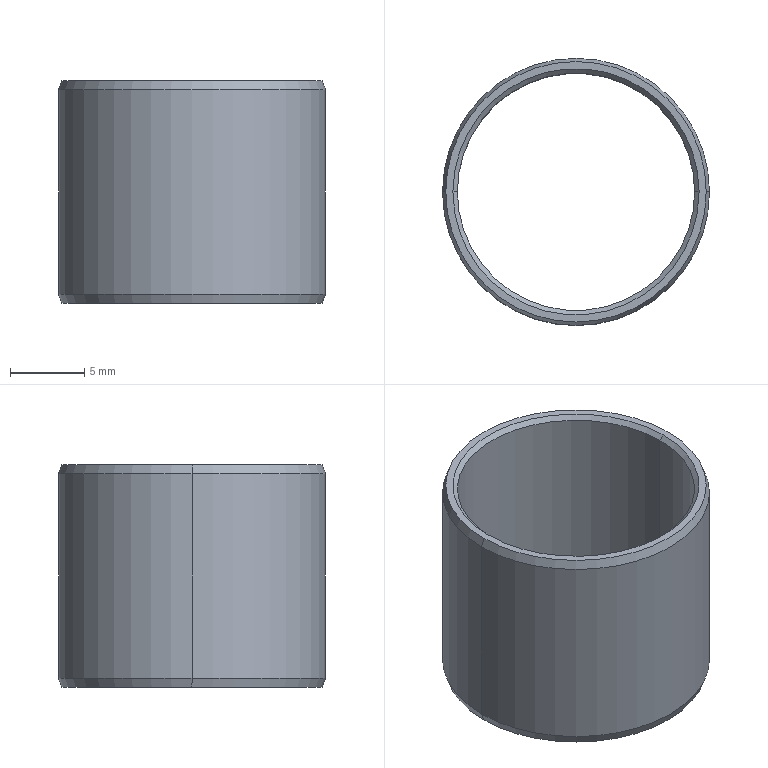Part | STEP file | SF-1 oil-free bearing 1615 | 1 solid | 14 faces | box 18 x 18 x 15 mm | volume 789.176 mm3 | cone 8 | cylinder 4 | plane 2 | commonest cylinder face diameters 16 x2 18 x2
STEP:
#1=CARTESIAN_POINT('',(0.,0.,0.));
#2=DIRECTION('',(0.,0.,1.));
#3=DIRECTION('',(1.,0.,0.));
#4=AXIS2_PLACEMENT_3D('',#1,#2,#3);
#5=CARTESIAN_POINT('',(-8.782,0.,0.));
#6=VERTEX_POINT('',#5);
#7=CARTESIAN_POINT('',(8.782,0.,0.));
#8=VERTEX_POINT('',#7);
#9=CARTESIAN_POINT('',(0.,0.,0.));
#10=DIRECTION('',(0.,0.,-1.));
#11=DIRECTION('',(1.,0.,0.));
#12=AXIS2_PLACEMENT_3D('',#9,#10,#11);
#13=CIRCLE('',#12,8.782);
#14=CARTESIAN_POINT('',(0.,0.,0.6));
#15=DIRECTION('',(0.,0.,1.));
#16=DIRECTION('',(1.,0.,0.));
#17=AXIS2_PLACEMENT_3D('',#14,#15,#16);
#18=CONICAL_SURFACE('',#17,9.,0.3491);
#19=CARTESIAN_POINT('',(6.283,-0.6));
#20=DIRECTION('',(-1.,0.));
#21=VECTOR('',#20,1.);
#22=LINE('',#19,#21);
#23=(GEOMETRIC_REPRESENTATION_CONTEXT(2)PARAMETRIC_REPRESENTATION_CONTEXT()REPRESENTATION_CONTEXT('',''));
#24=DEFINITIONAL_REPRESENTATION('',(#22),#23);
#25=PCURVE('',#18,#24);
#26=CARTESIAN_POINT('',(0.,0.,0.));
#27=DIRECTION('',(0.,0.,1.));
#28=DIRECTION('',(1.,0.,0.));
#29=AXIS2_PLACEMENT_3D('',#26,#27,#28);
#30=PLANE('',#29);
#31=CARTESIAN_POINT('',(8.782,0.));
#32=CARTESIAN_POINT('',(8.782,-15.21));
#33=CARTESIAN_POINT('',(-4.391,-7.605));
#34=CARTESIAN_POINT('',(-17.563,0.));
#35=CARTESIAN_POINT('',(-4.391,7.605));
#36=CARTESIAN_POINT('',(8.782,15.21));
#37=CARTESIAN_POINT('',(8.782,0.));
#38=(BOUNDED_CURVE()B_SPLINE_CURVE(2,(#31,#32,#33,#34,#35,#36,#37),.UNSPECIFIED.,.T.,.F.)B_SPLINE_CURVE_WITH_KNOTS((1,2,2,2,2,1),(-2.094,0.,2.094,4.189,6.283,8.378),.UNSPECIFIED.)CURVE()GEOMETRIC_REPRESENTATION_ITEM()RATIONAL_B_SPLINE_CURVE((1.,0.5,1.,0.5,1.,0.5,1.))REPRESENTATION_ITEM(''));
#39=(GEOMETRIC_REPRESENTATION_CONTEXT(2)PARAMETRIC_REPRESENTATION_CONTEXT()REPRESENTATION_CONTEXT('',''));
#40=DEFINITIONAL_REPRESENTATION('',(#38),#39);
#41=PCURVE('',#30,#40);
#42=SURFACE_CURVE('',#13,(#25,#41),.PCURVE_S1.);
#43=EDGE_CURVE('',#6,#8,#42,.T.);
#44=ORIENTED_EDGE('',*,*,#43,.F.);
#45=CARTESIAN_POINT('',(-9.,0.,0.6));
#46=VERTEX_POINT('',#45);
#47=CARTESIAN_POINT('',(-9.,0.,0.6));
#48=DIRECTION('',(-0.342,0.,0.9397));
#49=VECTOR('',#48,1.);
#50=LINE('',#47,#49);
#51=CARTESIAN_POINT('',(3.142,0.));
#52=DIRECTION('',(0.,1.));
#53=VECTOR('',#52,1.);
#54=LINE('',#51,#53);
#55=(GEOMETRIC_REPRESENTATION_CONTEXT(2)PARAMETRIC_REPRESENTATION_CONTEXT()REPRESENTATION_CONTEXT('',''));
#56=DEFINITIONAL_REPRESENTATION('',(#54),#55);
#57=PCURVE('',#18,#56);
#58=CARTESIAN_POINT('',(0.,0.,0.6));
#59=DIRECTION('',(0.,0.,1.));
#60=DIRECTION('',(1.,0.,0.));
#61=AXIS2_PLACEMENT_3D('',#58,#59,#60);
#62=CONICAL_SURFACE('',#61,9.,0.3491);
#63=CARTESIAN_POINT('',(3.142,0.));
#64=DIRECTION('',(0.,1.));
#65=VECTOR('',#64,1.);
#66=LINE('',#63,#65);
#67=(GEOMETRIC_REPRESENTATION_CONTEXT(2)PARAMETRIC_REPRESENTATION_CONTEXT()REPRESENTATION_CONTEXT('',''));
#68=DEFINITIONAL_REPRESENTATION('',(#66),#67);
#69=PCURVE('',#62,#68);
#70=SURFACE_CURVE('',#50,(#57,#69),.PCURVE_S1.);
#71=EDGE_CURVE('',#6,#46,#70,.T.);
#72=ORIENTED_EDGE('',*,*,#71,.T.);
#73=CARTESIAN_POINT('',(9.,0.,0.6));
#74=VERTEX_POINT('',#73);
#75=CARTESIAN_POINT('',(0.,0.,0.6));
#76=DIRECTION('',(0.,0.,1.));
#77=DIRECTION('',(1.,0.,0.));
#78=AXIS2_PLACEMENT_3D('',#75,#76,#77);
#79=CIRCLE('',#78,9.);
#80=CARTESIAN_POINT('',(0.,0.));
#81=DIRECTION('',(1.,0.));
#82=VECTOR('',#81,1.);
#83=LINE('',#80,#82);
#84=(GEOMETRIC_REPRESENTATION_CONTEXT(2)PARAMETRIC_REPRESENTATION_CONTEXT()REPRESENTATION_CONTEXT('',''));
#85=DEFINITIONAL_REPRESENTATION('',(#83),#84);
#86=PCURVE('',#18,#85);
#87=CARTESIAN_POINT('',(0.,0.,15.));
#88=DIRECTION('',(0.,0.,-1.));
#89=DIRECTION('',(-1.,0.,0.));
#90=AXIS2_PLACEMENT_3D('',#87,#88,#89);
#91=CYLINDRICAL_SURFACE('',#90,9.);
#92=CARTESIAN_POINT('',(3.142,14.4));
#93=DIRECTION('',(-1.,0.));
#94=VECTOR('',#93,1.);
#95=LINE('',#92,#94);
#96=(GEOMETRIC_REPRESENTATION_CONTEXT(2)PARAMETRIC_REPRESENTATION_CONTEXT()REPRESENTATION_CONTEXT('',''));
#97=DEFINITIONAL_REPRESENTATION('',(#95),#96);
#98=PCURVE('',#91,#97);
#99=SURFACE_CURVE('',#79,(#86,#98),.PCURVE_S1.);
#100=EDGE_CURVE('',#74,#46,#99,.T.);
#101=ORIENTED_EDGE('',*,*,#100,.F.);
#102=CARTESIAN_POINT('',(9.,0.,0.6));
#103=DIRECTION('',(0.342,0.,0.9397));
#104=VECTOR('',#103,1.);
#105=LINE('',#102,#104);
#106=CARTESIAN_POINT('',(0.,0.));
#107=DIRECTION('',(0.,1.));
#108=VECTOR('',#107,1.);
#109=LINE('',#106,#108);
#110=(GEOMETRIC_REPRESENTATION_CONTEXT(2)PARAMETRIC_REPRESENTATION_CONTEXT()REPRESENTATION_CONTEXT('',''));
#111=DEFINITIONAL_REPRESENTATION('',(#109),#110);
#112=PCURVE('',#18,#111);
#113=CARTESIAN_POINT('',(6.283,0.));
#114=DIRECTION('',(0.,1.));
#115=VECTOR('',#114,1.);
#116=LINE('',#113,#115);
#117=(GEOMETRIC_REPRESENTATION_CONTEXT(2)PARAMETRIC_REPRESENTATION_CONTEXT()REPRESENTATION_CONTEXT('',''));
#118=DEFINITIONAL_REPRESENTATION('',(#116),#117);
#119=PCURVE('',#62,#118);
#120=SURFACE_CURVE('',#105,(#112,#119),.PCURVE_S1.);
#121=EDGE_CURVE('',#8,#74,#120,.T.);
#122=ORIENTED_EDGE('',*,*,#121,.F.);
#123=EDGE_LOOP('',(#44,#72,#101,#122));
#124=FACE_BOUND('',#123,.T.);
#125=ADVANCED_FACE('',(#124),#18,.T.);
#126=CARTESIAN_POINT('',(8.782,0.,15.));
#127=VERTEX_POINT('',#126);
#128=CARTESIAN_POINT('',(-8.782,0.,15.));
#129=VERTEX_POINT('',#128);
#130=CARTESIAN_POINT('',(0.,0.,15.));
#131=DIRECTION('',(0.,0.,1.));
#132=DIRECTION('',(1.,0.,0.));
#133=AXIS2_PLACEMENT_3D('',#130,#131,#132);
#134=CIRCLE('',#133,8.782);
#135=CARTESIAN_POINT('',(0.,0.,15.));
#136=DIRECTION('',(0.,0.,-1.));
#137=DIRECTION('',(-1.,0.,0.));
#138=AXIS2_PLACEMENT_3D('',#135,#136,#137);
#139=CONICAL_SURFACE('',#138,8.782,0.3491);
#140=CARTESIAN_POINT('',(3.142,0.));
#141=DIRECTION('',(-1.,0.));
#142=VECTOR('',#141,1.);
#143=LINE('',#140,#142);
#144=(GEOMETRIC_REPRESENTATION_CONTEXT(2)PARAMETRIC_REPRESENTATION_CONTEXT()REPRESENTATION_CONTEXT('',''));
#145=DEFINITIONAL_REPRESENTATION('',(#143),#144);
#146=PCURVE('',#139,#145);
#147=CARTESIAN_POINT('',(0.,0.,15.));
#148=DIRECTION('',(0.,0.,1.));
#149=DIRECTION('',(1.,0.,0.));
#150=AXIS2_PLACEMENT_3D('',#147,#148,#149);
#151=PLANE('',#150);
#152=CARTESIAN_POINT('',(0.,0.));
#153=DIRECTION('',(1.,0.));
#154=AXIS2_PLACEMENT_2D('',#152,#153);
#155=CIRCLE('',#154,8.782);
#156=(GEOMETRIC_REPRESENTATION_CONTEXT(2)PARAMETRIC_REPRESENTATION_CONTEXT()REPRESENTATION_CONTEXT('',''));
#157=DEFINITIONAL_REPRESENTATION('',(#155),#156);
#158=PCURVE('',#151,#157);
#159=SURFACE_CURVE('',#134,(#146,#158),.PCURVE_S1.);
#160=EDGE_CURVE('',#127,#129,#159,.T.);
#161=ORIENTED_EDGE('',*,*,#160,.F.);
#162=CARTESIAN_POINT('',(9.,0.,14.4));
#163=VERTEX_POINT('',#162);
#164=CARTESIAN_POINT('',(8.782,0.,15.));
#165=DIRECTION('',(0.342,0.,-0.9397));
#166=VECTOR('',#165,1.);
#167=LINE('',#164,#166);
#168=CARTESIAN_POINT('',(3.142,0.));
#169=DIRECTION('',(0.,1.));
#170=VECTOR('',#169,1.);
#171=LINE('',#168,#170);
#172=(GEOMETRIC_REPRESENTATION_CONTEXT(2)PARAMETRIC_REPRESENTATION_CONTEXT()REPRESENTATION_CONTEXT('',''));
#173=DEFINITIONAL_REPRESENTATION('',(#171),#172);
#174=PCURVE('',#139,#173);
#175=CARTESIAN_POINT('',(0.,0.,15.));
#176=DIRECTION('',(0.,0.,-1.));
#177=DIRECTION('',(-1.,0.,0.));
#178=AXIS2_PLACEMENT_3D('',#175,#176,#177);
#179=CONICAL_SURFACE('',#178,8.782,0.3491);
#180=CARTESIAN_POINT('',(3.142,0.));
#181=DIRECTION('',(0.,1.));
#182=VECTOR('',#181,1.);
#183=LINE('',#180,#182);
#184=(GEOMETRIC_REPRESENTATION_CONTEXT(2)PARAMETRIC_REPRESENTATION_CONTEXT()REPRESENTATION_CONTEXT('',''));
#185=DEFINITIONAL_REPRESENTATION('',(#183),#184);
#186=PCURVE('',#179,#185);
#187=SURFACE_CURVE('',#167,(#174,#186),.PCURVE_S1.);
#188=EDGE_CURVE('',#127,#163,#187,.T.);
#189=ORIENTED_EDGE('',*,*,#188,.T.);
#190=CARTESIAN_POINT('',(-9.,0.,14.4));
#191=VERTEX_POINT('',#190);
#192=CARTESIAN_POINT('',(0.,0.,14.4));
#193=DIRECTION('',(0.,0.,-1.));
#194=DIRECTION('',(1.,0.,0.));
#195=AXIS2_PLACEMENT_3D('',#192,#193,#194);
#196=CIRCLE('',#195,9.);
#197=CARTESIAN_POINT('',(-3.142,0.6));
#198=DIRECTION('',(1.,0.));
#199=VECTOR('',#198,1.);
#200=LINE('',#197,#199);
#201=(GEOMETRIC_REPRESENTATION_CONTEXT(2)PARAMETRIC_REPRESENTATION_CONTEXT()REPRESENTATION_CONTEXT('',''));
#202=DEFINITIONAL_REPRESENTATION('',(#200),#201);
#203=PCURVE('',#139,#202);
#204=CARTESIAN_POINT('',(-3.142,0.6));
#205=DIRECTION('',(1.,0.));
#206=VECTOR('',#205,1.);
#207=LINE('',#204,#206);
#208=(GEOMETRIC_REPRESENTATION_CONTEXT(2)PARAMETRIC_REPRESENTATION_CONTEXT()REPRESENTATION_CONTEXT('',''));
#209=DEFINITIONAL_REPRESENTATION('',(#207),#208);
#210=PCURVE('',#91,#209);
#211=SURFACE_CURVE('',#196,(#203,#210),.PCURVE_S1.);
#212=EDGE_CURVE('',#191,#163,#211,.T.);
#213=ORIENTED_EDGE('',*,*,#212,.F.);
#214=CARTESIAN_POINT('',(-8.782,0.,15.));
#215=DIRECTION('',(-0.342,0.,-0.9397));
#216=VECTOR('',#215,1.);
#217=LINE('',#214,#216);
#218=CARTESIAN_POINT('',(0.,0.));
#219=DIRECTION('',(0.,1.));
#220=VECTOR('',#219,1.);
#221=LINE('',#218,#220);
#222=(GEOMETRIC_REPRESENTATION_CONTEXT(2)PARAMETRIC_REPRESENTATION_CONTEXT()REPRESENTATION_CONTEXT('',''));
#223=DEFINITIONAL_REPRESENTATION('',(#221),#222);
#224=PCURVE('',#139,#223);
#225=CARTESIAN_POINT('',(6.283,0.));
#226=DIRECTION('',(0.,1.));
#227=VECTOR('',#226,1.);
#228=LINE('',#225,#227);
#229=(GEOMETRIC_REPRESENTATION_CONTEXT(2)PARAMETRIC_REPRESENTATION_CONTEXT()REPRESENTATION_CONTEXT('',''));
#230=DEFINITIONAL_REPRESENTATION('',(#228),#229);
#231=PCURVE('',#179,#230);
#232=SURFACE_CURVE('',#217,(#224,#231),.PCURVE_S1.);
#233=EDGE_CURVE('',#129,#191,#232,.T.);
#234=ORIENTED_EDGE('',*,*,#233,.F.);
#235=EDGE_LOOP('',(#161,#189,#213,#234));
#236=FACE_BOUND('',#235,.T.);
#237=ADVANCED_FACE('',(#236),#139,.T.);
#238=CARTESIAN_POINT('',(8.,0.,14.7));
#239=VERTEX_POINT('',#238);
#240=CARTESIAN_POINT('',(8.3,0.,15.));
#241=VERTEX_POINT('',#240);
#242=CARTESIAN_POINT('',(8.,0.,14.7));
#243=DIRECTION('',(0.7071,0.,0.7071));
#244=VECTOR('',#243,1.);
#245=LINE('',#242,#244);
#246=CARTESIAN_POINT('',(0.,0.,14.7));
#247=DIRECTION('',(0.,0.,1.));
#248=DIRECTION('',(1.,0.,0.));
#249=AXIS2_PLACEMENT_3D('',#246,#247,#248);
#250=CONICAL_SURFACE('',#249,8.,0.7854);
#251=CARTESIAN_POINT('',(6.283,0.));
#252=DIRECTION('',(0.,1.));
#253=VECTOR('',#252,1.);
#254=LINE('',#251,#253);
#255=(GEOMETRIC_REPRESENTATION_CONTEXT(2)PARAMETRIC_REPRESENTATION_CONTEXT()REPRESENTATION_CONTEXT('',''));
#256=DEFINITIONAL_REPRESENTATION('',(#254),#255);
#257=PCURVE('',#250,#256);
#258=CARTESIAN_POINT('',(0.,0.,14.7));
#259=DIRECTION('',(0.,0.,1.));
#260=DIRECTION('',(1.,0.,0.));
#261=AXIS2_PLACEMENT_3D('',#258,#259,#260);
#262=CONICAL_SURFACE('',#261,8.,0.7854);
#263=CARTESIAN_POINT('',(0.,0.));
#264=DIRECTION('',(0.,1.));
#265=VECTOR('',#264,1.);
#266=LINE('',#263,#265);
#267=(GEOMETRIC_REPRESENTATION_CONTEXT(2)PARAMETRIC_REPRESENTATION_CONTEXT()REPRESENTATION_CONTEXT('',''));
#268=DEFINITIONAL_REPRESENTATION('',(#266),#267);
#269=PCURVE('',#262,#268);
#270=SURFACE_CURVE('',#245,(#257,#269),.PCURVE_S1.);
#271=EDGE_CURVE('',#239,#241,#270,.T.);
#272=ORIENTED_EDGE('',*,*,#271,.T.);
#273=CARTESIAN_POINT('',(-8.3,0.,15.));
#274=VERTEX_POINT('',#273);
#275=CARTESIAN_POINT('',(0.,0.,15.));
#276=DIRECTION('',(0.,0.,-1.));
#277=DIRECTION('',(1.,0.,0.));
#278=AXIS2_PLACEMENT_3D('',#275,#276,#277);
#279=CIRCLE('',#278,8.3);
#280=CARTESIAN_POINT('',(6.283,0.3));
#281=DIRECTION('',(-1.,0.));
#282=VECTOR('',#281,1.);
#283=LINE('',#280,#282);
#284=(GEOMETRIC_REPRESENTATION_CONTEXT(2)PARAMETRIC_REPRESENTATION_CONTEXT()REPRESENTATION_CONTEXT('',''));
#285=DEFINITIONAL_REPRESENTATION('',(#283),#284);
#286=PCURVE('',#250,#285);
#287=CARTESIAN_POINT('',(8.3,0.));
#288=CARTESIAN_POINT('',(8.3,-14.376));
#289=CARTESIAN_POINT('',(-4.15,-7.188));
#290=CARTESIAN_POINT('',(-16.6,0.));
#291=CARTESIAN_POINT('',(-4.15,7.188));
#292=CARTESIAN_POINT('',(8.3,14.376));
#293=CARTESIAN_POINT('',(8.3,0.));
#294=(BOUNDED_CURVE()B_SPLINE_CURVE(2,(#287,#288,#289,#290,#291,#292,#293),.UNSPECIFIED.,.T.,.F.)B_SPLINE_CURVE_WITH_KNOTS((1,2,2,2,2,1),(-2.094,0.,2.094,4.189,6.283,8.378),.UNSPECIFIED.)CURVE()GEOMETRIC_REPRESENTATION_ITEM()RATIONAL_B_SPLINE_CURVE((1.,0.5,1.,0.5,1.,0.5,1.))REPRESENTATION_ITEM(''));
#295=(GEOMETRIC_REPRESENTATION_CONTEXT(2)PARAMETRIC_REPRESENTATION_CONTEXT()REPRESENTATION_CONTEXT('',''));
#296=DEFINITIONAL_REPRESENTATION('',(#294),#295);
#297=PCURVE('',#151,#296);
#298=SURFACE_CURVE('',#279,(#286,#297),.PCURVE_S1.);
#299=EDGE_CURVE('',#241,#274,#298,.T.);
#300=ORIENTED_EDGE('',*,*,#299,.T.);
#301=CARTESIAN_POINT('',(-8.,0.,14.7));
#302=VERTEX_POINT('',#301);
#303=CARTESIAN_POINT('',(-8.,0.,14.7));
#304=DIRECTION('',(-0.7071,0.,0.7071));
#305=VECTOR('',#304,1.);
#306=LINE('',#303,#305);
#307=CARTESIAN_POINT('',(3.142,0.));
#308=DIRECTION('',(0.,1.));
#309=VECTOR('',#308,1.);
#310=LINE('',#307,#309);
#311=(GEOMETRIC_REPRESENTATION_CONTEXT(2)PARAMETRIC_REPRESENTATION_CONTEXT()REPRESENTATION_CONTEXT('',''));
#312=DEFINITIONAL_REPRESENTATION('',(#310),#311);
#313=PCURVE('',#250,#312);
#314=CARTESIAN_POINT('',(3.142,0.));
#315=DIRECTION('',(0.,1.));
#316=VECTOR('',#315,1.);
#317=LINE('',#314,#316);
#318=(GEOMETRIC_REPRESENTATION_CONTEXT(2)PARAMETRIC_REPRESENTATION_CONTEXT()REPRESENTATION_CONTEXT('',''));
#319=DEFINITIONAL_REPRESENTATION('',(#317),#318);
#320=PCURVE('',#262,#319);
#321=SURFACE_CURVE('',#306,(#313,#320),.PCURVE_S1.);
#322=EDGE_CURVE('',#302,#274,#321,.T.);
#323=ORIENTED_EDGE('',*,*,#322,.F.);
#324=CARTESIAN_POINT('',(0.,0.,14.7));
#325=DIRECTION('',(0.,0.,1.));
#326=DIRECTION('',(1.,0.,0.));
#327=AXIS2_PLACEMENT_3D('',#324,#325,#326);
#328=CIRCLE('',#327,8.);
#329=CARTESIAN_POINT('',(0.,0.));
#330=DIRECTION('',(1.,0.));
#331=VECTOR('',#330,1.);
#332=LINE('',#329,#331);
#333=(GEOMETRIC_REPRESENTATION_CONTEXT(2)PARAMETRIC_REPRESENTATION_CONTEXT()REPRESENTATION_CONTEXT('',''));
#334=DEFINITIONAL_REPRESENTATION('',(#332),#333);
#335=PCURVE('',#250,#334);
#336=CARTESIAN_POINT('',(0.,0.,15.));
#337=DIRECTION('',(0.,0.,-1.));
#338=DIRECTION('',(-1.,0.,0.));
#339=AXIS2_PLACEMENT_3D('',#336,#337,#338);
#340=CYLINDRICAL_SURFACE('',#339,8.);
#341=CARTESIAN_POINT('',(9.425,0.3));
#342=DIRECTION('',(-1.,0.));
#343=VECTOR('',#342,1.);
#344=LINE('',#341,#343);
#345=(GEOMETRIC_REPRESENTATION_CONTEXT(2)PARAMETRIC_REPRESENTATION_CONTEXT()REPRESENTATION_CONTEXT('',''));
#346=DEFINITIONAL_REPRESENTATION('',(#344),#345);
#347=PCURVE('',#340,#346);
#348=SURFACE_CURVE('',#328,(#335,#347),.PCURVE_S1.);
#349=EDGE_CURVE('',#302,#239,#348,.T.);
#350=ORIENTED_EDGE('',*,*,#349,.T.);
#351=EDGE_LOOP('',(#272,#300,#323,#350));
#352=FACE_BOUND('',#351,.F.);
#353=ADVANCED_FACE('',(#352),#250,.F.);
#354=CARTESIAN_POINT('',(-8.,0.,0.3));
#355=VERTEX_POINT('',#354);
#356=CARTESIAN_POINT('',(-8.3,0.,0.));
#357=VERTEX_POINT('',#356);
#358=CARTESIAN_POINT('',(-8.3,0.,0.));
#359=DIRECTION('',(-0.7071,0.,-0.7071));
#360=VECTOR('',#359,1.);
#361=LINE('',#358,#360);
#362=CARTESIAN_POINT('',(0.,0.,0.));
#363=DIRECTION('',(0.,0.,-1.));
#364=DIRECTION('',(-1.,0.,0.));
#365=AXIS2_PLACEMENT_3D('',#362,#363,#364);
#366=CONICAL_SURFACE('',#365,8.3,0.7854);
#367=CARTESIAN_POINT('',(6.283,0.));
#368=DIRECTION('',(0.,1.));
#369=VECTOR('',#368,1.);
#370=LINE('',#367,#369);
#371=(GEOMETRIC_REPRESENTATION_CONTEXT(2)PARAMETRIC_REPRESENTATION_CONTEXT()REPRESENTATION_CONTEXT('',''));
#372=DEFINITIONAL_REPRESENTATION('',(#370),#371);
#373=PCURVE('',#366,#372);
#374=CARTESIAN_POINT('',(0.,0.,0.));
#375=DIRECTION('',(0.,0.,-1.));
#376=DIRECTION('',(-1.,0.,0.));
#377=AXIS2_PLACEMENT_3D('',#374,#375,#376);
#378=CONICAL_SURFACE('',#377,8.3,0.7854);
#379=CARTESIAN_POINT('',(0.,0.));
#380=DIRECTION('',(0.,1.));
#381=VECTOR('',#380,1.);
#382=LINE('',#379,#381);
#383=(GEOMETRIC_REPRESENTATION_CONTEXT(2)PARAMETRIC_REPRESENTATION_CONTEXT()REPRESENTATION_CONTEXT('',''));
#384=DEFINITIONAL_REPRESENTATION('',(#382),#383);
#385=PCURVE('',#378,#384);
#386=SURFACE_CURVE('',#361,(#373,#385),.PCURVE_S1.);
#387=EDGE_CURVE('',#355,#357,#386,.T.);
#388=ORIENTED_EDGE('',*,*,#387,.T.);
#389=CARTESIAN_POINT('',(8.3,0.,0.));
#390=VERTEX_POINT('',#389);
#391=CARTESIAN_POINT('',(0.,0.,0.));
#392=DIRECTION('',(0.,0.,1.));
#393=DIRECTION('',(1.,0.,0.));
#394=AXIS2_PLACEMENT_3D('',#391,#392,#393);
#395=CIRCLE('',#394,8.3);
#396=CARTESIAN_POINT('',(9.425,0.));
#397=DIRECTION('',(-1.,0.));
#398=VECTOR('',#397,1.);
#399=LINE('',#396,#398);
#400=(GEOMETRIC_REPRESENTATION_CONTEXT(2)PARAMETRIC_REPRESENTATION_CONTEXT()REPRESENTATION_CONTEXT('',''));
#401=DEFINITIONAL_REPRESENTATION('',(#399),#400);
#402=PCURVE('',#366,#401);
#403=CARTESIAN_POINT('',(0.,0.));
#404=DIRECTION('',(1.,0.));
#405=AXIS2_PLACEMENT_2D('',#403,#404);
#406=CIRCLE('',#405,8.3);
#407=(GEOMETRIC_REPRESENTATION_CONTEXT(2)PARAMETRIC_REPRESENTATION_CONTEXT()REPRESENTATION_CONTEXT('',''));
#408=DEFINITIONAL_REPRESENTATION('',(#406),#407);
#409=PCURVE('',#30,#408);
#410=SURFACE_CURVE('',#395,(#402,#409),.PCURVE_S1.);
#411=EDGE_CURVE('',#357,#390,#410,.T.);
#412=ORIENTED_EDGE('',*,*,#411,.T.);
#413=CARTESIAN_POINT('',(8.,0.,0.3));
#414=VERTEX_POINT('',#413);
#415=CARTESIAN_POINT('',(8.3,0.,0.));
#416=DIRECTION('',(0.7071,0.,-0.7071));
#417=VECTOR('',#416,1.);
#418=LINE('',#415,#417);
#419=CARTESIAN_POINT('',(3.142,0.));
#420=DIRECTION('',(0.,1.));
#421=VECTOR('',#420,1.);
#422=LINE('',#419,#421);
#423=(GEOMETRIC_REPRESENTATION_CONTEXT(2)PARAMETRIC_REPRESENTATION_CONTEXT()REPRESENTATION_CONTEXT('',''));
#424=DEFINITIONAL_REPRESENTATION('',(#422),#423);
#425=PCURVE('',#366,#424);
#426=CARTESIAN_POINT('',(3.142,0.));
#427=DIRECTION('',(0.,1.));
#428=VECTOR('',#427,1.);
#429=LINE('',#426,#428);
#430=(GEOMETRIC_REPRESENTATION_CONTEXT(2)PARAMETRIC_REPRESENTATION_CONTEXT()REPRESENTATION_CONTEXT('',''));
#431=DEFINITIONAL_REPRESENTATION('',(#429),#430);
#432=PCURVE('',#378,#431);
#433=SURFACE_CURVE('',#418,(#425,#432),.PCURVE_S1.);
#434=EDGE_CURVE('',#414,#390,#433,.T.);
#435=ORIENTED_EDGE('',*,*,#434,.F.);
#436=CARTESIAN_POINT('',(0.,0.,0.3));
#437=DIRECTION('',(0.,0.,-1.));
#438=DIRECTION('',(1.,0.,0.));
#439=AXIS2_PLACEMENT_3D('',#436,#437,#438);
#440=CIRCLE('',#439,8.);
#441=CARTESIAN_POINT('',(3.142,-0.3));
#442=DIRECTION('',(1.,0.));
#443=VECTOR('',#442,1.);
#444=LINE('',#441,#443);
#445=(GEOMETRIC_REPRESENTATION_CONTEXT(2)PARAMETRIC_REPRESENTATION_CONTEXT()REPRESENTATION_CONTEXT('',''));
#446=DEFINITIONAL_REPRESENTATION('',(#444),#445);
#447=PCURVE('',#366,#446);
#448=CARTESIAN_POINT('',(3.142,14.7));
#449=DIRECTION('',(1.,0.));
#450=VECTOR('',#449,1.);
#451=LINE('',#448,#450);
#452=(GEOMETRIC_REPRESENTATION_CONTEXT(2)PARAMETRIC_REPRESENTATION_CONTEXT()REPRESENTATION_CONTEXT('',''));
#453=DEFINITIONAL_REPRESENTATION('',(#451),#452);
#454=PCURVE('',#340,#453);
#455=SURFACE_CURVE('',#440,(#447,#454),.PCURVE_S1.);
#456=EDGE_CURVE('',#414,#355,#455,.T.);
#457=ORIENTED_EDGE('',*,*,#456,.T.);
#458=EDGE_LOOP('',(#388,#412,#435,#457));
#459=FACE_BOUND('',#458,.F.);
#460=ADVANCED_FACE('',(#459),#366,.F.);
#461=CARTESIAN_POINT('',(-8.,0.,15.));
#462=DIRECTION('',(0.,0.,-1.));
#463=VECTOR('',#462,1.);
#464=LINE('',#461,#463);
#465=CARTESIAN_POINT('',(6.283,0.));
#466=DIRECTION('',(0.,1.));
#467=VECTOR('',#466,1.);
#468=LINE('',#465,#467);
#469=(GEOMETRIC_REPRESENTATION_CONTEXT(2)PARAMETRIC_REPRESENTATION_CONTEXT()REPRESENTATION_CONTEXT('',''));
#470=DEFINITIONAL_REPRESENTATION('',(#468),#469);
#471=PCURVE('',#340,#470);
#472=CARTESIAN_POINT('',(0.,0.,15.));
#473=DIRECTION('',(0.,0.,-1.));
#474=DIRECTION('',(-1.,0.,0.));
#475=AXIS2_PLACEMENT_3D('',#472,#473,#474);
#476=CYLINDRICAL_SURFACE('',#475,8.);
#477=CARTESIAN_POINT('',(0.,0.));
#478=DIRECTION('',(0.,1.));
#479=VECTOR('',#478,1.);
#480=LINE('',#477,#479);
#481=(GEOMETRIC_REPRESENTATION_CONTEXT(2)PARAMETRIC_REPRESENTATION_CONTEXT()REPRESENTATION_CONTEXT('',''));
#482=DEFINITIONAL_REPRESENTATION('',(#480),#481);
#483=PCURVE('',#476,#482);
#484=SURFACE_CURVE('',#464,(#471,#483),.PCURVE_S1.);
#485=EDGE_CURVE('',#302,#355,#484,.T.);
#486=ORIENTED_EDGE('',*,*,#485,.T.);
#487=ORIENTED_EDGE('',*,*,#456,.F.);
#488=CARTESIAN_POINT('',(8.,0.,15.));
#489=DIRECTION('',(0.,0.,-1.));
#490=VECTOR('',#489,1.);
#491=LINE('',#488,#490);
#492=CARTESIAN_POINT('',(3.142,0.));
#493=DIRECTION('',(0.,1.));
#494=VECTOR('',#493,1.);
#495=LINE('',#492,#494);
#496=(GEOMETRIC_REPRESENTATION_CONTEXT(2)PARAMETRIC_REPRESENTATION_CONTEXT()REPRESENTATION_CONTEXT('',''));
#497=DEFINITIONAL_REPRESENTATION('',(#495),#496);
#498=PCURVE('',#340,#497);
#499=CARTESIAN_POINT('',(3.142,0.));
#500=DIRECTION('',(0.,1.));
#501=VECTOR('',#500,1.);
#502=LINE('',#499,#501);
#503=(GEOMETRIC_REPRESENTATION_CONTEXT(2)PARAMETRIC_REPRESENTATION_CONTEXT()REPRESENTATION_CONTEXT('',''));
#504=DEFINITIONAL_REPRESENTATION('',(#502),#503);
#505=PCURVE('',#476,#504);
#506=SURFACE_CURVE('',#491,(#498,#505),.PCURVE_S1.);
#507=EDGE_CURVE('',#239,#414,#506,.T.);
#508=ORIENTED_EDGE('',*,*,#507,.F.);
#509=ORIENTED_EDGE('',*,*,#349,.F.);
#510=EDGE_LOOP('',(#486,#487,#508,#509));
#511=FACE_BOUND('',#510,.F.);
#512=ADVANCED_FACE('',(#511),#340,.F.);
#513=ORIENTED_EDGE('',*,*,#212,.T.);
#514=CARTESIAN_POINT('',(9.,0.,15.));
#515=DIRECTION('',(0.,0.,-1.));
#516=VECTOR('',#515,1.);
#517=LINE('',#514,#516);
#518=CARTESIAN_POINT('',(3.142,0.));
#519=DIRECTION('',(0.,1.));
#520=VECTOR('',#519,1.);
#521=LINE('',#518,#520);
#522=(GEOMETRIC_REPRESENTATION_CONTEXT(2)PARAMETRIC_REPRESENTATION_CONTEXT()REPRESENTATION_CONTEXT('',''));
#523=DEFINITIONAL_REPRESENTATION('',(#521),#522);
#524=PCURVE('',#91,#523);
#525=CARTESIAN_POINT('',(0.,0.,15.));
#526=DIRECTION('',(0.,0.,-1.));
#527=DIRECTION('',(-1.,0.,0.));
#528=AXIS2_PLACEMENT_3D('',#525,#526,#527);
#529=CYLINDRICAL_SURFACE('',#528,9.);
#530=CARTESIAN_POINT('',(3.142,0.));
#531=DIRECTION('',(0.,1.));
#532=VECTOR('',#531,1.);
#533=LINE('',#530,#532);
#534=(GEOMETRIC_REPRESENTATION_CONTEXT(2)PARAMETRIC_REPRESENTATION_CONTEXT()REPRESENTATION_CONTEXT('',''));
#535=DEFINITIONAL_REPRESENTATION('',(#533),#534);
#536=PCURVE('',#529,#535);
#537=SURFACE_CURVE('',#517,(#524,#536),.PCURVE_S1.);
#538=EDGE_CURVE('',#163,#74,#537,.T.);
#539=ORIENTED_EDGE('',*,*,#538,.T.);
#540=ORIENTED_EDGE('',*,*,#100,.T.);
#541=CARTESIAN_POINT('',(-9.,0.,15.));
#542=DIRECTION('',(0.,0.,-1.));
#543=VECTOR('',#542,1.);
#544=LINE('',#541,#543);
#545=CARTESIAN_POINT('',(0.,0.));
#546=DIRECTION('',(0.,1.));
#547=VECTOR('',#546,1.);
#548=LINE('',#545,#547);
#549=(GEOMETRIC_REPRESENTATION_CONTEXT(2)PARAMETRIC_REPRESENTATION_CONTEXT()REPRESENTATION_CONTEXT('',''));
#550=DEFINITIONAL_REPRESENTATION('',(#548),#549);
#551=PCURVE('',#91,#550);
#552=CARTESIAN_POINT('',(6.283,0.));
#553=DIRECTION('',(0.,1.));
#554=VECTOR('',#553,1.);
#555=LINE('',#552,#554);
#556=(GEOMETRIC_REPRESENTATION_CONTEXT(2)PARAMETRIC_REPRESENTATION_CONTEXT()REPRESENTATION_CONTEXT('',''));
#557=DEFINITIONAL_REPRESENTATION('',(#555),#556);
#558=PCURVE('',#529,#557);
#559=SURFACE_CURVE('',#544,(#551,#558),.PCURVE_S1.);
#560=EDGE_CURVE('',#191,#46,#559,.T.);
#561=ORIENTED_EDGE('',*,*,#560,.F.);
#562=EDGE_LOOP('',(#513,#539,#540,#561));
#563=FACE_BOUND('',#562,.T.);
#564=ADVANCED_FACE('',(#563),#91,.T.);
#565=CARTESIAN_POINT('',(0.,0.,15.));
#566=DIRECTION('',(0.,0.,1.));
#567=DIRECTION('',(1.,0.,0.));
#568=AXIS2_PLACEMENT_3D('',#565,#566,#567);
#569=CIRCLE('',#568,8.782);
#570=CARTESIAN_POINT('',(0.,0.));
#571=DIRECTION('',(1.,0.));
#572=AXIS2_PLACEMENT_2D('',#570,#571);
#573=CIRCLE('',#572,8.782);
#574=(GEOMETRIC_REPRESENTATION_CONTEXT(2)PARAMETRIC_REPRESENTATION_CONTEXT()REPRESENTATION_CONTEXT('',''));
#575=DEFINITIONAL_REPRESENTATION('',(#573),#574);
#576=PCURVE('',#151,#575);
#577=CARTESIAN_POINT('',(9.425,0.));
#578=DIRECTION('',(-1.,0.));
#579=VECTOR('',#578,1.);
#580=LINE('',#577,#579);
#581=(GEOMETRIC_REPRESENTATION_CONTEXT(2)PARAMETRIC_REPRESENTATION_CONTEXT()REPRESENTATION_CONTEXT('',''));
#582=DEFINITIONAL_REPRESENTATION('',(#580),#581);
#583=PCURVE('',#179,#582);
#584=SURFACE_CURVE('',#569,(#576,#583),.PCURVE_S1.);
#585=EDGE_CURVE('',#129,#127,#584,.T.);
#586=ORIENTED_EDGE('',*,*,#585,.T.);
#587=ORIENTED_EDGE('',*,*,#160,.T.);
#588=EDGE_LOOP('',(#586,#587));
#589=FACE_BOUND('',#588,.T.);
#590=ORIENTED_EDGE('',*,*,#299,.T.);
#591=CARTESIAN_POINT('',(0.,0.,15.));
#592=DIRECTION('',(0.,0.,-1.));
#593=DIRECTION('',(1.,0.,0.));
#594=AXIS2_PLACEMENT_3D('',#591,#592,#593);
#595=CIRCLE('',#594,8.3);
#596=CARTESIAN_POINT('',(8.3,0.));
#597=CARTESIAN_POINT('',(8.3,-14.376));
#598=CARTESIAN_POINT('',(-4.15,-7.188));
#599=CARTESIAN_POINT('',(-16.6,0.));
#600=CARTESIAN_POINT('',(-4.15,7.188));
#601=CARTESIAN_POINT('',(8.3,14.376));
#602=CARTESIAN_POINT('',(8.3,0.));
#603=(BOUNDED_CURVE()B_SPLINE_CURVE(2,(#596,#597,#598,#599,#600,#601,#602),.UNSPECIFIED.,.T.,.F.)B_SPLINE_CURVE_WITH_KNOTS((1,2,2,2,2,1),(-2.094,0.,2.094,4.189,6.283,8.378),.UNSPECIFIED.)CURVE()GEOMETRIC_REPRESENTATION_ITEM()RATIONAL_B_SPLINE_CURVE((1.,0.5,1.,0.5,1.,0.5,1.))REPRESENTATION_ITEM(''));
#604=(GEOMETRIC_REPRESENTATION_CONTEXT(2)PARAMETRIC_REPRESENTATION_CONTEXT()REPRESENTATION_CONTEXT('',''));
#605=DEFINITIONAL_REPRESENTATION('',(#603),#604);
#606=PCURVE('',#151,#605);
#607=CARTESIAN_POINT('',(6.283,0.3));
#608=DIRECTION('',(-1.,0.));
#609=VECTOR('',#608,1.);
#610=LINE('',#607,#609);
#611=(GEOMETRIC_REPRESENTATION_CONTEXT(2)PARAMETRIC_REPRESENTATION_CONTEXT()REPRESENTATION_CONTEXT('',''));
#612=DEFINITIONAL_REPRESENTATION('',(#610),#611);
#613=PCURVE('',#262,#612);
#614=SURFACE_CURVE('',#595,(#606,#613),.PCURVE_S1.);
#615=EDGE_CURVE('',#274,#241,#614,.T.);
#616=ORIENTED_EDGE('',*,*,#615,.T.);
#617=EDGE_LOOP('',(#590,#616));
#618=FACE_BOUND('',#617,.T.);
#619=ADVANCED_FACE('',(#589,#618),#151,.T.);
#620=CARTESIAN_POINT('',(0.,0.,0.));
#621=DIRECTION('',(0.,0.,-1.));
#622=DIRECTION('',(1.,0.,0.));
#623=AXIS2_PLACEMENT_3D('',#620,#621,#622);
#624=CIRCLE('',#623,8.782);
#625=CARTESIAN_POINT('',(8.782,0.));
#626=CARTESIAN_POINT('',(8.782,-15.21));
#627=CARTESIAN_POINT('',(-4.391,-7.605));
#628=CARTESIAN_POINT('',(-17.563,0.));
#629=CARTESIAN_POINT('',(-4.391,7.605));
#630=CARTESIAN_POINT('',(8.782,15.21));
#631=CARTESIAN_POINT('',(8.782,0.));
#632=(BOUNDED_CURVE()B_SPLINE_CURVE(2,(#625,#626,#627,#628,#629,#630,#631),.UNSPECIFIED.,.T.,.F.)B_SPLINE_CURVE_WITH_KNOTS((1,2,2,2,2,1),(-2.094,0.,2.094,4.189,6.283,8.378),.UNSPECIFIED.)CURVE()GEOMETRIC_REPRESENTATION_ITEM()RATIONAL_B_SPLINE_CURVE((1.,0.5,1.,0.5,1.,0.5,1.))REPRESENTATION_ITEM(''));
#633=(GEOMETRIC_REPRESENTATION_CONTEXT(2)PARAMETRIC_REPRESENTATION_CONTEXT()REPRESENTATION_CONTEXT('',''));
#634=DEFINITIONAL_REPRESENTATION('',(#632),#633);
#635=PCURVE('',#30,#634);
#636=CARTESIAN_POINT('',(6.283,-0.6));
#637=DIRECTION('',(-1.,0.));
#638=VECTOR('',#637,1.);
#639=LINE('',#636,#638);
#640=(GEOMETRIC_REPRESENTATION_CONTEXT(2)PARAMETRIC_REPRESENTATION_CONTEXT()REPRESENTATION_CONTEXT('',''));
#641=DEFINITIONAL_REPRESENTATION('',(#639),#640);
#642=PCURVE('',#62,#641);
#643=SURFACE_CURVE('',#624,(#635,#642),.PCURVE_S1.);
#644=EDGE_CURVE('',#8,#6,#643,.T.);
#645=ORIENTED_EDGE('',*,*,#644,.T.);
#646=ORIENTED_EDGE('',*,*,#43,.T.);
#647=EDGE_LOOP('',(#645,#646));
#648=FACE_BOUND('',#647,.T.);
#649=ORIENTED_EDGE('',*,*,#411,.T.);
#650=CARTESIAN_POINT('',(0.,0.,0.));
#651=DIRECTION('',(0.,0.,1.));
#652=DIRECTION('',(1.,0.,0.));
#653=AXIS2_PLACEMENT_3D('',#650,#651,#652);
#654=CIRCLE('',#653,8.3);
#655=CARTESIAN_POINT('',(0.,0.));
#656=DIRECTION('',(1.,0.));
#657=AXIS2_PLACEMENT_2D('',#655,#656);
#658=CIRCLE('',#657,8.3);
#659=(GEOMETRIC_REPRESENTATION_CONTEXT(2)PARAMETRIC_REPRESENTATION_CONTEXT()REPRESENTATION_CONTEXT('',''));
#660=DEFINITIONAL_REPRESENTATION('',(#658),#659);
#661=PCURVE('',#30,#660);
#662=CARTESIAN_POINT('',(3.142,0.));
#663=DIRECTION('',(-1.,0.));
#664=VECTOR('',#663,1.);
#665=LINE('',#662,#664);
#666=(GEOMETRIC_REPRESENTATION_CONTEXT(2)PARAMETRIC_REPRESENTATION_CONTEXT()REPRESENTATION_CONTEXT('',''));
#667=DEFINITIONAL_REPRESENTATION('',(#665),#666);
#668=PCURVE('',#378,#667);
#669=SURFACE_CURVE('',#654,(#661,#668),.PCURVE_S1.);
#670=EDGE_CURVE('',#390,#357,#669,.T.);
#671=ORIENTED_EDGE('',*,*,#670,.T.);
#672=EDGE_LOOP('',(#649,#671));
#673=FACE_BOUND('',#672,.T.);
#674=ADVANCED_FACE('',(#648,#673),#30,.F.);
#675=ORIENTED_EDGE('',*,*,#538,.F.);
#676=CARTESIAN_POINT('',(0.,0.,14.4));
#677=DIRECTION('',(0.,0.,-1.));
#678=DIRECTION('',(1.,0.,0.));
#679=AXIS2_PLACEMENT_3D('',#676,#677,#678);
#680=CIRCLE('',#679,9.);
#681=CARTESIAN_POINT('',(3.142,0.6));
#682=DIRECTION('',(1.,0.));
#683=VECTOR('',#682,1.);
#684=LINE('',#681,#683);
#685=(GEOMETRIC_REPRESENTATION_CONTEXT(2)PARAMETRIC_REPRESENTATION_CONTEXT()REPRESENTATION_CONTEXT('',''));
#686=DEFINITIONAL_REPRESENTATION('',(#684),#685);
#687=PCURVE('',#529,#686);
#688=CARTESIAN_POINT('',(3.142,0.6));
#689=DIRECTION('',(1.,0.));
#690=VECTOR('',#689,1.);
#691=LINE('',#688,#690);
#692=(GEOMETRIC_REPRESENTATION_CONTEXT(2)PARAMETRIC_REPRESENTATION_CONTEXT()REPRESENTATION_CONTEXT('',''));
#693=DEFINITIONAL_REPRESENTATION('',(#691),#692);
#694=PCURVE('',#179,#693);
#695=SURFACE_CURVE('',#680,(#687,#694),.PCURVE_S1.);
#696=EDGE_CURVE('',#163,#191,#695,.T.);
#697=ORIENTED_EDGE('',*,*,#696,.T.);
#698=ORIENTED_EDGE('',*,*,#560,.T.);
#699=CARTESIAN_POINT('',(0.,0.,0.6));
#700=DIRECTION('',(0.,0.,1.));
#701=DIRECTION('',(1.,0.,0.));
#702=AXIS2_PLACEMENT_3D('',#699,#700,#701);
#703=CIRCLE('',#702,9.);
#704=CARTESIAN_POINT('',(9.425,14.4));
#705=DIRECTION('',(-1.,0.));
#706=VECTOR('',#705,1.);
#707=LINE('',#704,#706);
#708=(GEOMETRIC_REPRESENTATION_CONTEXT(2)PARAMETRIC_REPRESENTATION_CONTEXT()REPRESENTATION_CONTEXT('',''));
#709=DEFINITIONAL_REPRESENTATION('',(#707),#708);
#710=PCURVE('',#529,#709);
#711=CARTESIAN_POINT('',(0.,0.));
#712=DIRECTION('',(1.,0.));
#713=VECTOR('',#712,1.);
#714=LINE('',#711,#713);
#715=(GEOMETRIC_REPRESENTATION_CONTEXT(2)PARAMETRIC_REPRESENTATION_CONTEXT()REPRESENTATION_CONTEXT('',''));
#716=DEFINITIONAL_REPRESENTATION('',(#714),#715);
#717=PCURVE('',#62,#716);
#718=SURFACE_CURVE('',#703,(#710,#717),.PCURVE_S1.);
#719=EDGE_CURVE('',#46,#74,#718,.T.);
#720=ORIENTED_EDGE('',*,*,#719,.T.);
#721=EDGE_LOOP('',(#675,#697,#698,#720));
#722=FACE_BOUND('',#721,.T.);
#723=ADVANCED_FACE('',(#722),#529,.T.);
#724=CARTESIAN_POINT('',(0.,0.,0.3));
#725=DIRECTION('',(0.,0.,-1.));
#726=DIRECTION('',(1.,0.,0.));
#727=AXIS2_PLACEMENT_3D('',#724,#725,#726);
#728=CIRCLE('',#727,8.);
#729=CARTESIAN_POINT('',(-3.142,14.7));
#730=DIRECTION('',(1.,0.));
#731=VECTOR('',#730,1.);
#732=LINE('',#729,#731);
#733=(GEOMETRIC_REPRESENTATION_CONTEXT(2)PARAMETRIC_REPRESENTATION_CONTEXT()REPRESENTATION_CONTEXT('',''));
#734=DEFINITIONAL_REPRESENTATION('',(#732),#733);
#735=PCURVE('',#476,#734);
#736=CARTESIAN_POINT('',(-3.142,-0.3));
#737=DIRECTION('',(1.,0.));
#738=VECTOR('',#737,1.);
#739=LINE('',#736,#738);
#740=(GEOMETRIC_REPRESENTATION_CONTEXT(2)PARAMETRIC_REPRESENTATION_CONTEXT()REPRESENTATION_CONTEXT('',''));
#741=DEFINITIONAL_REPRESENTATION('',(#739),#740);
#742=PCURVE('',#378,#741);
#743=SURFACE_CURVE('',#728,(#735,#742),.PCURVE_S1.);
#744=EDGE_CURVE('',#355,#414,#743,.T.);
#745=ORIENTED_EDGE('',*,*,#744,.F.);
#746=ORIENTED_EDGE('',*,*,#485,.F.);
#747=CARTESIAN_POINT('',(0.,0.,14.7));
#748=DIRECTION('',(0.,0.,1.));
#749=DIRECTION('',(1.,0.,0.));
#750=AXIS2_PLACEMENT_3D('',#747,#748,#749);
#751=CIRCLE('',#750,8.);
#752=CARTESIAN_POINT('',(3.142,0.3));
#753=DIRECTION('',(-1.,0.));
#754=VECTOR('',#753,1.);
#755=LINE('',#752,#754);
#756=(GEOMETRIC_REPRESENTATION_CONTEXT(2)PARAMETRIC_REPRESENTATION_CONTEXT()REPRESENTATION_CONTEXT('',''));
#757=DEFINITIONAL_REPRESENTATION('',(#755),#756);
#758=PCURVE('',#476,#757);
#759=CARTESIAN_POINT('',(0.,0.));
#760=DIRECTION('',(1.,0.));
#761=VECTOR('',#760,1.);
#762=LINE('',#759,#761);
#763=(GEOMETRIC_REPRESENTATION_CONTEXT(2)PARAMETRIC_REPRESENTATION_CONTEXT()REPRESENTATION_CONTEXT('',''));
#764=DEFINITIONAL_REPRESENTATION('',(#762),#763);
#765=PCURVE('',#262,#764);
#766=SURFACE_CURVE('',#751,(#758,#765),.PCURVE_S1.);
#767=EDGE_CURVE('',#239,#302,#766,.T.);
#768=ORIENTED_EDGE('',*,*,#767,.F.);
#769=ORIENTED_EDGE('',*,*,#507,.T.);
#770=EDGE_LOOP('',(#745,#746,#768,#769));
#771=FACE_BOUND('',#770,.F.);
#772=ADVANCED_FACE('',(#771),#476,.F.);
#773=ORIENTED_EDGE('',*,*,#670,.T.);
#774=ORIENTED_EDGE('',*,*,#387,.F.);
#775=ORIENTED_EDGE('',*,*,#744,.T.);
#776=ORIENTED_EDGE('',*,*,#434,.T.);
#777=EDGE_LOOP('',(#773,#774,#775,#776));
#778=FACE_BOUND('',#777,.F.);
#779=ADVANCED_FACE('',(#778),#378,.F.);
#780=ORIENTED_EDGE('',*,*,#615,.T.);
#781=ORIENTED_EDGE('',*,*,#271,.F.);
#782=ORIENTED_EDGE('',*,*,#767,.T.);
#783=ORIENTED_EDGE('',*,*,#322,.T.);
#784=EDGE_LOOP('',(#780,#781,#782,#783));
#785=FACE_BOUND('',#784,.F.);
#786=ADVANCED_FACE('',(#785),#262,.F.);
#787=ORIENTED_EDGE('',*,*,#188,.F.);
#788=ORIENTED_EDGE('',*,*,#585,.F.);
#789=ORIENTED_EDGE('',*,*,#233,.T.);
#790=ORIENTED_EDGE('',*,*,#696,.F.);
#791=EDGE_LOOP('',(#787,#788,#789,#790));
#792=FACE_BOUND('',#791,.T.);
#793=ADVANCED_FACE('',(#792),#179,.T.);
#794=ORIENTED_EDGE('',*,*,#71,.F.);
#795=ORIENTED_EDGE('',*,*,#644,.F.);
#796=ORIENTED_EDGE('',*,*,#121,.T.);
#797=ORIENTED_EDGE('',*,*,#719,.F.);
#798=EDGE_LOOP('',(#794,#795,#796,#797));
#799=FACE_BOUND('',#798,.T.);
#800=ADVANCED_FACE('',(#799),#62,.T.);
#801=CLOSED_SHELL('',(#125,#237,#353,#460,#512,#564,#619,#674,#723,#772,#779,#786,#793,#800));
#802=MANIFOLD_SOLID_BREP('',#801);
#803=(LENGTH_UNIT()NAMED_UNIT(*)SI_UNIT(.MILLI.,.METRE.));
#804=UNCERTAINTY_MEASURE_WITH_UNIT(LENGTH_MEASURE(0.0000001),#803,'','');
#805=(NAMED_UNIT(*)PLANE_ANGLE_UNIT()SI_UNIT($,.RADIAN.));
#806=(NAMED_UNIT(*)SI_UNIT($,.STERADIAN.)SOLID_ANGLE_UNIT());
#807=(GEOMETRIC_REPRESENTATION_CONTEXT(3)GLOBAL_UNCERTAINTY_ASSIGNED_CONTEXT((#804))GLOBAL_UNIT_ASSIGNED_CONTEXT((#803,#805,#806))REPRESENTATION_CONTEXT('',''));
#808=ADVANCED_BREP_SHAPE_REPRESENTATION('',(#4,#802),#807);